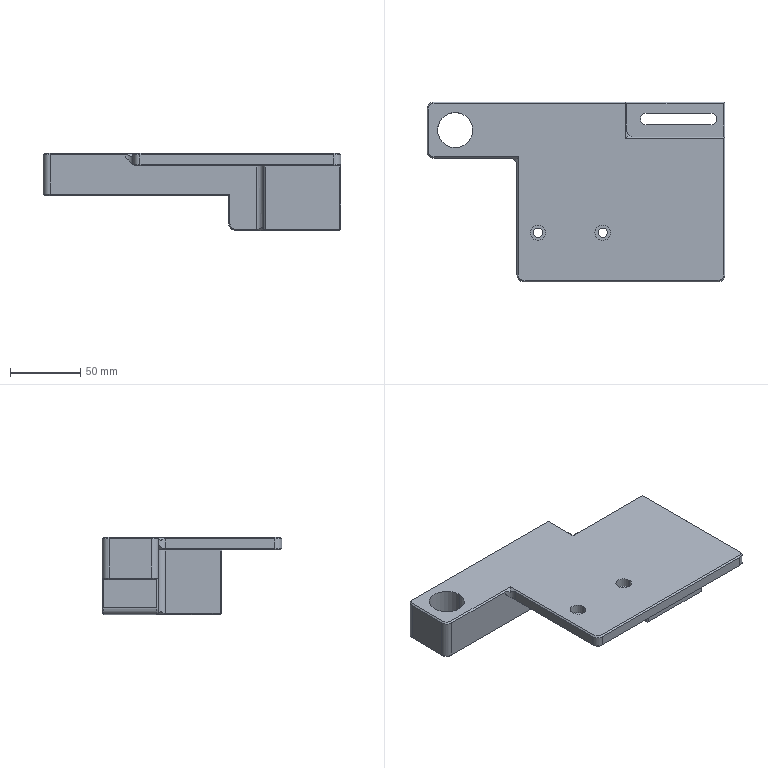NC program | NX | posted with a generic post | part box 212 x 128 x 55 mm
Lines 4578 to 5530 of 8014:
(ZLEVEL_PROFILE_COPY_COPY_COPY_COPY_1 , TOOL : D10)
N9136 T09 M6
N9138 G54
N9140 G17 G0 G90 X-41.719 Y17.8 S2000 M3
N9142 G43 Z30. H9
N9144 Z-0.2
N9146 G94 G1 X-42.585 Y19.3 F1000.
N9148 G3 X-43.451 Y19.8 R1.
N9150 G1 X-46.8 F2000.
N9152 Y16.451
N9154 G3 X-46.3 Y15.585 R1.
N9156 G1 X-44.8 Y14.719
N9158 G0 X-41.519 Y17.6 Z-0.4
N9160 G1 X-42.385 Y19.1 F1000.
N9162 G3 X-43.251 Y19.6 R1.
N9164 G1 X-46.6 F2000.
N9166 Y16.251
N9168 G3 X-46.1 Y15.385 R1.
N9170 G1 X-44.6 Y14.519
N9172 G0 X-41.319 Y17.4 Z-0.6
N9174 G1 X-42.185 Y18.9 F1000.
N9176 G3 X-43.051 Y19.4 R1.
N9178 G1 X-46.4 F2000.
N9180 Y16.051
N9182 G3 X-45.9 Y15.185 R1.
N9184 G1 X-44.4 Y14.319
N9186 G0 X-41.119 Y17.2 Z-0.8
N9188 G1 X-41.985 Y18.7 F1000.
N9190 G3 X-42.851 Y19.2 R1.
N9192 G1 X-46.2 F2000.
N9194 Y15.851
N9196 G3 X-45.7 Y14.985 R1.
N9198 G1 X-44.2 Y14.119
N9200 G0 X-40.919 Y17. Z-1.
N9202 G1 X-41.785 Y18.5 F1000.
N9204 G3 X-42.651 Y19. R1.
N9206 G1 X-45.559 F2000.
N9208 X-46.
N9210 Y15.651
N9212 G3 X-45.5 Y14.785 R1.
N9214 G1 X-44. Y13.919
N9216 G0 X-40.919 Y17. Z-1.2
N9218 G1 X-41.785 Y18.5 F1000.
N9220 G3 X-42.651 Y19. R1.
N9222 G1 X-45.997 F2000.
N9224 X-46. Y18.997
N9226 Y15.651
N9228 G3 X-45.5 Y14.785 R1.
N9230 G1 X-44. Y13.919
N9232 G0 X-40.919 Y17. Z-1.4
N9234 G1 X-41.785 Y18.5 F1000.
N9236 G3 X-42.651 Y19. R1.
N9238 G1 X-45.997 F2000.
N9240 X-46. Y18.997
N9242 Y15.651
N9244 G3 X-45.5 Y14.785 R1.
N9246 G1 X-44. Y13.919
N9248 G0 X-40.919 Y17. Z-1.6
N9250 G1 X-41.785 Y18.5 F1000.
N9252 G3 X-42.651 Y19. R1.
N9254 G1 X-45.997 F2000.
N9256 X-46. Y18.997
N9258 Y15.651
N9260 G3 X-45.5 Y14.785 R1.
N9262 G1 X-44. Y13.919
N9264 G0 X-40.919 Y17. Z-1.8
N9266 G1 X-41.785 Y18.5 F1000.
N9268 G3 X-42.651 Y19. R1.
N9270 G1 X-45.997 F2000.
N9272 X-46. Y18.997
N9274 Y15.651
N9276 G3 X-45.5 Y14.785 R1.
N9278 G1 X-44. Y13.919
N9280 G0 X-40.919 Y17. Z-2.
N9282 G1 X-41.785 Y18.5 F1000.
N9284 G3 X-42.651 Y19. R1.
N9286 G1 X-45.997 F2000.
N9288 X-46. Y18.997
N9290 Y15.651
N9292 G3 X-45.5 Y14.785 R1.
N9294 G1 X-44. Y13.919
N9296 G0 X-40.919 Y17. Z-2.2
N9298 G1 X-41.785 Y18.5 F1000.
N9300 G3 X-42.651 Y19. R1.
N9302 G1 X-45.997 F2000.
N9304 X-46. Y18.997
N9306 Y15.651
N9308 G3 X-45.5 Y14.785 R1.
N9310 G1 X-44. Y13.919
N9312 G0 X-40.919 Y17. Z-2.4
N9314 G1 X-41.785 Y18.5 F1000.
N9316 G3 X-42.651 Y19. R1.
N9318 G1 X-45.997 F2000.
N9320 X-46. Y18.997
N9322 Y15.651
N9324 G3 X-45.5 Y14.785 R1.
N9326 G1 X-44. Y13.919
N9328 G0 X-40.919 Y17. Z-2.6
N9330 G1 X-41.785 Y18.5 F1000.
N9332 G3 X-42.651 Y19. R1.
N9334 G1 X-45.997 F2000.
N9336 X-46. Y18.997
N9338 Y15.651
N9340 G3 X-45.5 Y14.785 R1.
N9342 G1 X-44. Y13.919
N9344 G0 X-40.919 Y17. Z-2.8
N9346 G1 X-41.785 Y18.5 F1000.
N9348 G3 X-42.651 Y19. R1.
N9350 G1 X-45.997 F2000.
N9352 X-46. Y18.997
N9354 Y15.651
N9356 G3 X-45.5 Y14.785 R1.
N9358 G1 X-44. Y13.919
N9360 G0 X-40.919 Y17. Z-3.
N9362 G1 X-41.785 Y18.5 F1000.
N9364 G3 X-42.651 Y19. R1.
N9366 G1 X-45.997 F2000.
N9368 X-46. Y18.997
N9370 Y15.651
N9372 G3 X-45.5 Y14.785 R1.
N9374 G1 X-44. Y13.919
N9376 G0 X-40.919 Y17. Z-3.2
N9378 G1 X-41.785 Y18.5 F1000.
N9380 G3 X-42.651 Y19. R1.
N9382 G1 X-45.997 F2000.
N9384 X-46. Y18.997
N9386 Y15.651
N9388 G3 X-45.5 Y14.785 R1.
N9390 G1 X-44. Y13.919
N9392 G0 X-40.919 Y17. Z-3.4
N9394 G1 X-41.785 Y18.5 F1000.
N9396 G3 X-42.651 Y19. R1.
N9398 G1 X-45.997 F2000.
N9400 X-46. Y18.997
N9402 Y15.651
N9404 G3 X-45.5 Y14.785 R1.
N9406 G1 X-44. Y13.919
N9408 G0 X-40.919 Y17. Z-3.6
N9410 G1 X-41.785 Y18.5 F1000.
N9412 G3 X-42.651 Y19. R1.
N9414 G1 X-45.997 F2000.
N9416 X-46. Y18.997
N9418 Y15.651
N9420 G3 X-45.5 Y14.785 R1.
N9422 G1 X-44. Y13.919
N9424 G0 X-40.919 Y17. Z-3.8
N9426 G1 X-41.785 Y18.5 F1000.
N9428 G3 X-42.651 Y19. R1.
N9430 G1 X-45.997 F2000.
N9432 X-46. Y18.997
N9434 Y15.651
N9436 G3 X-45.5 Y14.785 R1.
N9438 G1 X-44. Y13.919
N9440 G0 X-40.919 Y17. Z-4.
N9442 G1 X-41.785 Y18.5 F1000.
N9444 G3 X-42.651 Y19. R1.
N9446 G1 X-45.997 F2000.
N9448 X-46. Y18.997
N9450 Y15.651
N9452 G3 X-45.5 Y14.785 R1.
N9454 G1 X-44. Y13.919
N9456 G0 X-40.919 Y17. Z-4.2
N9458 G1 X-41.785 Y18.5 F1000.
N9460 G3 X-42.651 Y19. R1.
N9462 G1 X-45.997 F2000.
N9464 X-46. Y18.997
N9466 Y15.651
N9468 G3 X-45.5 Y14.785 R1.
N9470 G1 X-44. Y13.919
N9472 G0 X-40.919 Y17. Z-4.4
N9474 G1 X-41.785 Y18.5 F1000.
N9476 G3 X-42.651 Y19. R1.
N9478 G1 X-45.997 F2000.
N9480 X-46. Y18.997
N9482 Y15.651
N9484 G3 X-45.5 Y14.785 R1.
N9486 G1 X-44. Y13.919
N9488 G0 X-40.919 Y17. Z-4.6
N9490 G1 X-41.785 Y18.5 F1000.
N9492 G3 X-42.651 Y19. R1.
N9494 G1 X-45.997 F2000.
N9496 X-46. Y18.997
N9498 Y15.651
N9500 G3 X-45.5 Y14.785 R1.
N9502 G1 X-44. Y13.919
N9504 G0 X-40.919 Y17. Z-4.8
N9506 G1 X-41.785 Y18.5 F1000.
N9508 G3 X-42.651 Y19. R1.
N9510 G1 X-45.997 F2000.
N9512 X-46. Y18.997
N9514 Y15.651
N9516 G3 X-45.5 Y14.785 R1.
N9518 G1 X-44. Y13.919
N9520 G0 X-40.919 Y17. Z-5.
N9522 G1 X-41.785 Y18.5 F1000.
N9524 G3 X-42.651 Y19. R1.
N9526 G1 X-45.997 F2000.
N9528 X-46. Y18.997
N9530 Y15.651
N9532 G3 X-45.5 Y14.785 R1.
N9534 G1 X-44. Y13.919
N9536 G0 X-40.919 Y17. Z-5.2
N9538 G1 X-41.785 Y18.5 F1000.
N9540 G3 X-42.651 Y19. R1.
N9542 G1 X-45.997 F2000.
N9544 X-46. Y18.997
N9546 Y15.651
N9548 G3 X-45.5 Y14.785 R1.
N9550 G1 X-44. Y13.919
N9552 G0 X-40.919 Y17. Z-5.4
N9554 G1 X-41.785 Y18.5 F1000.
N9556 G3 X-42.651 Y19. R1.
N9558 G1 X-45.997 F2000.
N9560 X-46. Y18.997
N9562 Y15.651
N9564 G3 X-45.5 Y14.785 R1.
N9566 G1 X-44. Y13.919
N9568 G0 X-40.919 Y17. Z-5.6
N9570 G1 X-41.785 Y18.5 F1000.
N9572 G3 X-42.651 Y19. R1.
N9574 G1 X-45.997 F2000.
N9576 X-46. Y18.997
N9578 Y15.651
N9580 G3 X-45.5 Y14.785 R1.
N9582 G1 X-44. Y13.919
N9584 G0 X-40.919 Y17. Z-5.8
N9586 G1 X-41.785 Y18.5 F1000.
N9588 G3 X-42.651 Y19. R1.
N9590 G1 X-45.997 F2000.
N9592 X-46. Y18.997
N9594 Y15.651
N9596 G3 X-45.5 Y14.785 R1.
N9598 G1 X-44. Y13.919
N9600 G0 X-40.919 Y17. Z-6.
N9602 G1 X-41.785 Y18.5 F1000.
N9604 G3 X-42.651 Y19. R1.
N9606 G1 X-45.996 F2000.
N9608 X-46. Y18.996
N9610 Y15.651
N9612 G3 X-45.5 Y14.785 R1.
N9614 G1 X-44. Y13.919
N9616 G0 X-40.919 Y17. Z-6.2
N9618 G1 X-41.785 Y18.5 F1000.
N9620 G3 X-42.651 Y19. R1.
N9622 G1 X-45.996 F2000.
N9624 X-46. Y18.996
N9626 Y15.651
N9628 G3 X-45.5 Y14.785 R1.
N9630 G1 X-44. Y13.919
N9632 G0 X-40.919 Y17. Z-6.4
N9634 G1 X-41.785 Y18.5 F1000.
N9636 G3 X-42.651 Y19. R1.
N9638 G1 X-45.996 F2000.
N9640 X-46. Y18.996
N9642 Y15.651
N9644 G3 X-45.5 Y14.785 R1.
N9646 G1 X-44. Y13.919
N9648 G0 X-40.919 Y17. Z-6.6
N9650 G1 X-41.785 Y18.5 F1000.
N9652 G3 X-42.651 Y19. R1.
N9654 G1 X-45.996 F2000.
N9656 X-46. Y18.996
N9658 Y15.651
N9660 G3 X-45.5 Y14.785 R1.
N9662 G1 X-44. Y13.919
N9664 G0 X-40.919 Y17. Z-6.8
N9666 G1 X-41.785 Y18.5 F1000.
N9668 G3 X-42.651 Y19. R1.
N9670 G1 X-45.996 F2000.
N9672 X-46. Y18.996
N9674 Y15.651
N9676 G3 X-45.5 Y14.785 R1.
N9678 G1 X-44. Y13.919
N9680 G0 X-40.919 Y17. Z-7.
N9682 G1 X-41.785 Y18.5 F1000.
N9684 G3 X-42.651 Y19. R1.
N9686 G1 X-45.996 F2000.
N9688 X-46. Y18.996
N9690 Y15.651
N9692 G3 X-45.5 Y14.785 R1.
N9694 G1 X-44. Y13.919
N9696 G0 X-40.919 Y17. Z-7.2
N9698 G1 X-41.785 Y18.5 F1000.
N9700 G3 X-42.651 Y19. R1.
N9702 G1 X-45.996 F2000.
N9704 X-46. Y18.996
N9706 Y15.651
N9708 G3 X-45.5 Y14.785 R1.
N9710 G1 X-44. Y13.919
N9712 G0 X-40.919 Y17. Z-7.4
N9714 G1 X-41.785 Y18.5 F1000.
N9716 G3 X-42.651 Y19. R1.
N9718 G1 X-45.996 F2000.
N9720 X-46. Y18.996
N9722 Y15.651
N9724 G3 X-45.5 Y14.785 R1.
N9726 G1 X-44. Y13.919
N9728 G0 X-40.919 Y17. Z-7.6
N9730 G1 X-41.785 Y18.5 F1000.
N9732 G3 X-42.651 Y19. R1.
N9734 G1 X-45.996 F2000.
N9736 X-46. Y18.996
N9738 Y15.651
N9740 G3 X-45.5 Y14.785 R1.
N9742 G1 X-44. Y13.919
N9744 G0 X-40.919 Y17. Z-7.8
N9746 G1 X-41.785 Y18.5 F1000.
N9748 G3 X-42.651 Y19. R1.
N9750 G1 X-45.996 F2000.
N9752 X-46. Y18.996
N9754 Y15.651
N9756 G3 X-45.5 Y14.785 R1.
N9758 G1 X-44. Y13.919
N9760 G0 X-40.919 Y17. Z-8.
N9762 G1 X-41.785 Y18.5 F1000.
N9764 G3 X-42.651 Y19. R1.
N9766 G1 X-45.996 F2000.
N9768 X-46. Y18.996
N9770 Y15.651
N9772 G3 X-45.5 Y14.785 R1.
N9774 G1 X-44. Y13.919
N9776 G0 X-40.919 Y17. Z-8.2
N9778 G1 X-41.785 Y18.5 F1000.
N9780 G3 X-42.651 Y19. R1.
N9782 G1 X-45.996 F2000.
N9784 X-46. Y18.996
N9786 Y15.651
N9788 G3 X-45.5 Y14.785 R1.
N9790 G1 X-44. Y13.919
N9792 G0 X-40.919 Y17. Z-8.4
N9794 G1 X-41.785 Y18.5 F1000.
N9796 G3 X-42.651 Y19. R1.
N9798 G1 X-45.996 F2000.
N9800 X-46. Y18.996
N9802 Y15.651
N9804 G3 X-45.5 Y14.785 R1.
N9806 G1 X-44. Y13.919
N9808 G0 X-40.919 Y17. Z-8.6
N9810 G1 X-41.785 Y18.5 F1000.
N9812 G3 X-42.651 Y19. R1.
N9814 G1 X-45.996 F2000.
N9816 X-46. Y18.996
N9818 Y15.651
N9820 G3 X-45.5 Y14.785 R1.
N9822 G1 X-44. Y13.919
N9824 G0 X-40.919 Y17. Z-8.8
N9826 G1 X-41.785 Y18.5 F1000.
N9828 G3 X-42.651 Y19. R1.
N9830 G1 X-45.996 F2000.
N9832 X-46. Y18.996
N9834 Y15.651
N9836 G3 X-45.5 Y14.785 R1.
N9838 G1 X-44. Y13.919
N9840 G0 X-40.919 Y17. Z-9.
N9842 G1 X-41.785 Y18.5 F1000.
N9844 G3 X-42.651 Y19. R1.
N9846 G1 X-45.996 F2000.
N9848 X-46. Y18.996
N9850 Y15.651
N9852 G3 X-45.5 Y14.785 R1.
N9854 G1 X-44. Y13.919
N9856 G0 X-40.919 Y17. Z-9.2
N9858 G1 X-41.785 Y18.5 F1000.
N9860 G3 X-42.651 Y19. R1.
N9862 G1 X-45.996 F2000.
N9864 X-46. Y18.996
N9866 Y15.651
N9868 G3 X-45.5 Y14.785 R1.
N9870 G1 X-44. Y13.919
N9872 G0 X-40.919 Y17. Z-9.4
N9874 G1 X-41.785 Y18.5 F1000.
N9876 G3 X-42.651 Y19. R1.
N9878 G1 X-45.996 F2000.
N9880 X-46. Y18.996
N9882 Y15.651
N9884 G3 X-45.5 Y14.785 R1.
N9886 G1 X-44. Y13.919
N9888 G0 X-40.919 Y17. Z-9.6
N9890 G1 X-41.785 Y18.5 F1000.
N9892 G3 X-42.651 Y19. R1.
N9894 G1 X-45.996 F2000.
N9896 X-46. Y18.996
N9898 Y15.651
N9900 G3 X-45.5 Y14.785 R1.
N9902 G1 X-44. Y13.919
N9904 G0 X-40.919 Y17. Z-9.8
N9906 G1 X-41.785 Y18.5 F1000.
N9908 G3 X-42.651 Y19. R1.
N9910 G1 X-45.996 F2000.
N9912 X-46. Y18.996
N9914 Y15.651
N9916 G3 X-45.5 Y14.785 R1.
N9918 G1 X-44. Y13.919
N9920 G0 X-40.919 Y17. Z-10.
N9922 G1 X-41.785 Y18.5 F1000.
N9924 G3 X-42.651 Y19. R1.
N9926 G1 X-45.996 F2000.
N9928 X-46. Y18.996
N9930 Y15.651
N9932 G3 X-45.5 Y14.785 R1.
N9934 G1 X-44. Y13.919
N9936 G0 X-40.919 Y17. Z-10.2
N9938 G1 X-41.785 Y18.5 F1000.
N9940 G3 X-42.651 Y19. R1.
N9942 G1 X-45.996 F2000.
N9944 X-46. Y18.996
N9946 Y15.651
N9948 G3 X-45.5 Y14.785 R1.
N9950 G1 X-44. Y13.919
N9952 G0 X-40.919 Y17. Z-10.4
N9954 G1 X-41.785 Y18.5 F1000.
N9956 G3 X-42.651 Y19. R1.
N9958 G1 X-45.996 F2000.
N9960 X-46. Y18.996
N9962 Y15.651
N9964 G3 X-45.5 Y14.785 R1.
N9966 G1 X-44. Y13.919
N9968 G0 X-40.919 Y17. Z-10.6
N9970 G1 X-41.785 Y18.5 F1000.
N9972 G3 X-42.651 Y19. R1.
N9974 G1 X-45.996 F2000.
N9976 X-46. Y18.996
N9978 Y15.651
N9980 G3 X-45.5 Y14.785 R1.
N9982 G1 X-44. Y13.919
N9984 G0 X-40.919 Y17. Z-10.8
N9986 G1 X-41.785 Y18.5 F1000.
N9988 G3 X-42.651 Y19. R1.
N9990 G1 X-45.996 F2000.
N9992 X-46. Y18.996
N9994 Y15.651
N9996 G3 X-45.5 Y14.785 R1.
N9998 G1 X-44. Y13.919
N10000 G0 X-40.919 Y17. Z-11.
N10002 G1 X-41.785 Y18.5 F1000.
N10004 G3 X-42.651 Y19. R1.
N10006 G1 X-45.996 F2000.
N10008 X-46. Y18.996
N10010 Y15.651
N10012 G3 X-45.5 Y14.785 R1.
N10014 G1 X-44. Y13.919
N10016 G0 X-40.919 Y17. Z-11.2
N10018 G1 X-41.785 Y18.5 F1000.
N10020 G3 X-42.651 Y19. R1.
N10022 G1 X-45.996 F2000.
N10024 X-46. Y18.996
N10026 Y15.651
N10028 G3 X-45.5 Y14.785 R1.
N10030 G1 X-44. Y13.919
N10032 G0 X-40.919 Y17. Z-11.4
N10034 G1 X-41.785 Y18.5 F1000.
N10036 G3 X-42.651 Y19. R1.
N10038 G1 X-45.996 F2000.
N10040 X-46. Y18.996
N10042 Y15.651
N10044 G3 X-45.5 Y14.785 R1.
N10046 G1 X-44. Y13.919
N10048 G0 X-40.919 Y17. Z-11.6
N10050 G1 X-41.785 Y18.5 F1000.
N10052 G3 X-42.651 Y19. R1.
N10054 G1 X-45.996 F2000.
N10056 X-46. Y18.996
N10058 Y15.651
N10060 G3 X-45.5 Y14.785 R1.
N10062 G1 X-44. Y13.919
N10064 G0 X-40.919 Y17. Z-11.8
N10066 G1 X-41.785 Y18.5 F1000.
N10068 G3 X-42.651 Y19. R1.
N10070 G1 X-45.996 F2000.
N10072 X-46. Y18.996
N10074 Y15.651
N10076 G3 X-45.5 Y14.785 R1.
N10078 G1 X-44. Y13.919
N10080 G0 X-40.919 Y17. Z-12.
N10082 G1 X-41.785 Y18.5 F1000.
N10084 G3 X-42.651 Y19. R1.
N10086 G1 X-45.996 F2000.
N10088 X-46. Y18.996
N10090 Y15.651
N10092 G3 X-45.5 Y14.785 R1.
N10094 G1 X-44. Y13.919
N10096 G0 X-40.919 Y17. Z-12.2
N10098 G1 X-41.785 Y18.5 F1000.
N10100 G3 X-42.651 Y19. R1.
N10102 G1 X-45.996 F2000.
N10104 X-46. Y18.996
N10106 Y15.651
N10108 G3 X-45.5 Y14.785 R1.
N10110 G1 X-44. Y13.919
N10112 G0 X-40.919 Y17. Z-12.4
N10114 G1 X-41.785 Y18.5 F1000.
N10116 G3 X-42.651 Y19. R1.
N10118 G1 X-45.996 F2000.
N10120 X-46. Y18.996
N10122 Y15.651
N10124 G3 X-45.5 Y14.785 R1.
N10126 G1 X-44. Y13.919
N10128 G0 X-40.919 Y17. Z-12.6
N10130 G1 X-41.785 Y18.5 F1000.
N10132 G3 X-42.651 Y19. R1.
N10134 G1 X-45.996 F2000.
N10136 X-46. Y18.996
N10138 Y15.651
N10140 G3 X-45.5 Y14.785 R1.
N10142 G1 X-44. Y13.919
N10144 G0 X-40.919 Y17. Z-12.8
N10146 G1 X-41.785 Y18.5 F1000.
N10148 G3 X-42.651 Y19. R1.
N10150 G1 X-45.996 F2000.
N10152 X-46. Y18.996
N10154 Y15.651
N10156 G3 X-45.5 Y14.785 R1.
N10158 G1 X-44. Y13.919
N10160 G0 X-40.919 Y17. Z-13.
N10162 G1 X-41.785 Y18.5 F1000.
N10164 G3 X-42.651 Y19. R1.
N10166 G1 X-45.996 F2000.
N10168 X-46. Y18.996
N10170 Y15.651
N10172 G3 X-45.5 Y14.785 R1.
N10174 G1 X-44. Y13.919
N10176 G0 X-40.919 Y17. Z-13.2
N10178 G1 X-41.785 Y18.5 F1000.
N10180 G3 X-42.651 Y19. R1.
N10182 G1 X-45.996 F2000.
N10184 X-46. Y18.996
N10186 Y15.651
N10188 G3 X-45.5 Y14.785 R1.
N10190 G1 X-44. Y13.919
N10192 G0 X-40.919 Y17. Z-13.4
N10194 G1 X-41.785 Y18.5 F1000.
N10196 G3 X-42.651 Y19. R1.
N10198 G1 X-45.996 F2000.
N10200 X-46. Y18.996
N10202 Y15.651
N10204 G3 X-45.5 Y14.785 R1.
N10206 G1 X-44. Y13.919
N10208 G0 X-40.919 Y17. Z-13.6
N10210 G1 X-41.785 Y18.5 F1000.
N10212 G3 X-42.651 Y19. R1.
N10214 G1 X-45.996 F2000.
N10216 X-46. Y18.996
N10218 Y15.651
N10220 G3 X-45.5 Y14.785 R1.
N10222 G1 X-44. Y13.919
N10224 G0 X-40.919 Y17. Z-13.8
N10226 G1 X-41.785 Y18.5 F1000.
N10228 G3 X-42.651 Y19. R1.
N10230 G1 X-45.996 F2000.
N10232 X-46. Y18.996
N10234 Y15.651
N10236 G3 X-45.5 Y14.785 R1.
N10238 G1 X-44. Y13.919
N10240 G0 X-40.919 Y17. Z-14.
N10242 G1 X-41.785 Y18.5 F1000.
N10244 G3 X-42.651 Y19. R1.
N10246 G1 X-45.996 F2000.
N10248 X-46. Y18.996
N10250 Y15.651
N10252 G3 X-45.5 Y14.785 R1.
N10254 G1 X-44. Y13.919
N10256 G0 X-40.919 Y17. Z-14.2
N10258 G1 X-41.785 Y18.5 F1000.
N10260 G3 X-42.651 Y19. R1.
N10262 G1 X-45.996 F2000.
N10264 X-46. Y18.996
N10266 Y15.651
N10268 G3 X-45.5 Y14.785 R1.
N10270 G1 X-44. Y13.919
N10272 G0 X-40.919 Y17. Z-14.4
N10274 G1 X-41.785 Y18.5 F1000.
N10276 G3 X-42.651 Y19. R1.
N10278 G1 X-45.996 F2000.
N10280 X-46. Y18.996
N10282 Y15.651
N10284 G3 X-45.5 Y14.785 R1.
N10286 G1 X-44. Y13.919
N10288 G0 X-40.919 Y17. Z-14.6
N10290 G1 X-41.785 Y18.5 F1000.
N10292 G3 X-42.651 Y19. R1.
N10294 G1 X-45.996 F2000.
N10296 X-46. Y18.996
N10298 Y15.651
N10300 G3 X-45.5 Y14.785 R1.
N10302 G1 X-44. Y13.919
N10304 G0 X-40.919 Y17. Z-14.8
N10306 G1 X-41.785 Y18.5 F1000.
N10308 G3 X-42.651 Y19. R1.
N10310 G1 X-45.996 F2000.
N10312 X-46. Y18.996
N10314 Y15.651
N10316 G3 X-45.5 Y14.785 R1.
N10318 G1 X-44. Y13.919
N10320 G0 X-40.919 Y17. Z-15.
N10322 G1 X-41.785 Y18.5 F1000.
N10324 G3 X-42.651 Y19. R1.
N10326 G1 X-45.996 F2000.
N10328 X-46. Y18.996
N10330 Y15.651
N10332 G3 X-45.5 Y14.785 R1.
N10334 G1 X-44. Y13.919
N10336 G0 X-40.919 Y17. Z-15.2
N10338 G1 X-41.785 Y18.5 F1000.
N10340 G3 X-42.651 Y19. R1.
N10342 G1 X-45.996 F2000.
N10344 X-46. Y18.996
N10346 Y15.651
N10348 G3 X-45.5 Y14.785 R1.
N10350 G1 X-44. Y13.919
N10352 G0 X-40.919 Y17. Z-15.4
N10354 G1 X-41.785 Y18.5 F1000.
N10356 G3 X-42.651 Y19. R1.
N10358 G1 X-45.996 F2000.
N10360 X-46. Y18.996
N10362 Y15.651
N10364 G3 X-45.5 Y14.785 R1.
N10366 G1 X-44. Y13.919
N10368 G0 X-40.919 Y17. Z-15.6
N10370 G1 X-41.785 Y18.5 F1000.
N10372 G3 X-42.651 Y19. R1.
N10374 G1 X-45.996 F2000.
N10376 X-46. Y18.996
N10378 Y15.651
N10380 G3 X-45.5 Y14.785 R1.
N10382 G1 X-44. Y13.919
N10384 G0 X-40.919 Y17. Z-15.8
N10386 G1 X-41.785 Y18.5 F1000.
N10388 G3 X-42.651 Y19. R1.
N10390 G1 X-45.996 F2000.
N10392 X-46. Y18.996
N10394 Y15.651
N10396 G3 X-45.5 Y14.785 R1.
N10398 G1 X-44. Y13.919
N10400 G0 X-40.919 Y17. Z-16.
N10402 G1 X-41.785 Y18.5 F1000.
N10404 G3 X-42.651 Y19. R1.
N10406 G1 X-45.996 F2000.
N10408 X-46. Y18.996
N10410 Y15.651
N10412 G3 X-45.5 Y14.785 R1.
N10414 G1 X-44. Y13.919
N10416 G0 X-40.919 Y17. Z-16.2
N10418 G1 X-41.785 Y18.5 F1000.
N10420 G3 X-42.651 Y19. R1.
N10422 G1 X-45.996 F2000.
N10424 X-46. Y18.996
N10426 Y15.651
N10428 G3 X-45.5 Y14.785 R1.
N10430 G1 X-44. Y13.919
N10432 G0 X-40.919 Y17. Z-16.4
N10434 G1 X-41.785 Y18.5 F1000.
N10436 G3 X-42.651 Y19. R1.
N10438 G1 X-45.996 F2000.
N10440 X-46. Y18.996
N10442 Y15.651
N10444 G3 X-45.5 Y14.785 R1.
N10446 G1 X-44. Y13.919
N10448 G0 X-40.919 Y17. Z-16.6
N10450 G1 X-41.785 Y18.5 F1000.
N10452 G3 X-42.651 Y19. R1.
N10454 G1 X-45.996 F2000.
N10456 X-46. Y18.996
N10458 Y15.651
N10460 G3 X-45.5 Y14.785 R1.
N10462 G1 X-44. Y13.919
N10464 G0 X-40.919 Y17. Z-16.8
N10466 G1 X-41.785 Y18.5 F1000.
N10468 G3 X-42.651 Y19. R1.
N10470 G1 X-45.996 F2000.
N10472 X-46. Y18.996
N10474 Y15.651
N10476 G3 X-45.5 Y14.785 R1.
N10478 G1 X-44. Y13.919
N10480 G0 X-40.919 Y17. Z-17.
N10482 G1 X-41.785 Y18.5 F1000.
N10484 G3 X-42.651 Y19. R1.
N10486 G1 X-45.996 F2000.
N10488 X-46. Y18.996
N10490 Y15.651
N10492 G3 X-45.5 Y14.785 R1.
N10494 G1 X-44. Y13.919
N10496 G0 X-40.919 Y17. Z-17.2
N10498 G1 X-41.785 Y18.5 F1000.
N10500 G3 X-42.651 Y19. R1.
N10502 G1 X-45.996 F2000.
N10504 X-46. Y18.996
N10506 Y15.651
N10508 G3 X-45.5 Y14.785 R1.
N10510 G1 X-44. Y13.919
N10512 G0 X-40.919 Y17. Z-17.4
N10514 G1 X-41.785 Y18.5 F1000.
N10516 G3 X-42.651 Y19. R1.
N10518 G1 X-45.996 F2000.
N10520 X-46. Y18.996
N10522 Y15.651
N10524 G3 X-45.5 Y14.785 R1.
N10526 G1 X-44. Y13.919
N10528 G0 X-40.919 Y17. Z-17.6
N10530 G1 X-41.785 Y18.5 F1000.
N10532 G3 X-42.651 Y19. R1.
N10534 G1 X-45.996 F2000.
N10536 X-46. Y18.996
N10538 Y15.651
N10540 G3 X-45.5 Y14.785 R1.
N10542 G1 X-44. Y13.919
N10544 G0 X-40.919 Y17. Z-17.8
N10546 G1 X-41.785 Y18.5 F1000.
N10548 G3 X-42.651 Y19. R1.
N10550 G1 X-45.996 F2000.
N10552 X-46. Y18.996
N10554 Y15.651
N10556 G3 X-45.5 Y14.785 R1.
N10558 G1 X-44. Y13.919
N10560 G0 X-40.919 Y17. Z-18.
N10562 G1 X-41.785 Y18.5 F1000.
N10564 G3 X-42.651 Y19. R1.
N10566 G1 X-45.996 F2000.
N10568 X-46. Y18.996
N10570 Y15.651
N10572 G3 X-45.5 Y14.785 R1.
N10574 G1 X-44. Y13.919
N10576 G0 X-40.919 Y17. Z-18.2
N10578 G1 X-41.785 Y18.5 F1000.
N10580 G3 X-42.651 Y19. R1.
N10582 G1 X-45.996 F2000.
N10584 X-46. Y18.996
N10586 Y15.651
N10588 G3 X-45.5 Y14.785 R1.
N10590 G1 X-44. Y13.919
N10592 G0 X-40.919 Y17. Z-18.4
N10594 G1 X-41.785 Y18.5 F1000.
N10596 G3 X-42.651 Y19. R1.
N10598 G1 X-45.996 F2000.
N10600 X-46. Y18.996
N10602 Y15.651
N10604 G3 X-45.5 Y14.785 R1.
N10606 G1 X-44. Y13.919
N10608 G0 X-40.919 Y17. Z-18.6
N10610 G1 X-41.785 Y18.5 F1000.
N10612 G3 X-42.651 Y19. R1.
N10614 G1 X-45.996 F2000.
N10616 X-46. Y18.996
N10618 Y15.651
N10620 G3 X-45.5 Y14.785 R1.
N10622 G1 X-44. Y13.919
N10624 G0 X-40.919 Y17. Z-18.8
N10626 G1 X-41.785 Y18.5 F1000.
N10628 G3 X-42.651 Y19. R1.
N10630 G1 X-45.996 F2000.
N10632 X-46. Y18.996
N10634 Y15.651
N10636 G3 X-45.5 Y14.785 R1.
N10638 G1 X-44. Y13.919
N10640 G0 X-40.919 Y17. Z-19.
N10642 G1 X-41.785 Y18.5 F1000.
N10644 G3 X-42.651 Y19. R1.
N10646 G1 X-45.996 F2000.
N10648 X-46. Y18.996
N10650 Y15.651
N10652 G3 X-45.5 Y14.785 R1.
N10654 G1 X-44. Y13.919
N10656 G0 X-40.919 Y17. Z-19.2
N10658 G1 X-41.785 Y18.5 F1000.
N10660 G3 X-42.651 Y19. R1.
N10662 G1 X-45.996 F2000.
N10664 X-46. Y18.996
N10666 Y15.651
N10668 G3 X-45.5 Y14.785 R1.
N10670 G1 X-44. Y13.919
N10672 G0 X-40.919 Y17. Z-19.4
N10674 G1 X-41.785 Y18.5 F1000.
N10676 G3 X-42.651 Y19. R1.
N10678 G1 X-45.996 F2000.
N10680 X-46. Y18.996
N10682 Y15.651
N10684 G3 X-45.5 Y14.785 R1.
N10686 G1 X-44. Y13.919
N10688 G0 X-40.919 Y17. Z-19.6
N10690 G1 X-41.785 Y18.5 F1000.
N10692 G3 X-42.651 Y19. R1.
N10694 G1 X-45.996 F2000.
N10696 X-46. Y18.996
N10698 Y15.651
N10700 G3 X-45.5 Y14.785 R1.
N10702 G1 X-44. Y13.919
N10704 G0 X-40.919 Y17. Z-19.8
N10706 G1 X-41.785 Y18.5 F1000.
N10708 G3 X-42.651 Y19. R1.
N10710 G1 X-45.996 F2000.
N10712 X-46. Y18.996
N10714 Y15.651
N10716 G3 X-45.5 Y14.785 R1.
N10718 G1 X-44. Y13.919
N10720 G0 X-40.919 Y17. Z-20.
N10722 G1 X-41.785 Y18.5 F1000.
N10724 G3 X-42.651 Y19. R1.
N10726 G1 X-45.996 F2000.
N10728 X-46. Y18.996
N10730 Y15.651
N10732 G3 X-45.5 Y14.785 R1.
N10734 G1 X-44. Y13.919
N10736 G0 X-40.919 Y17. Z-20.2
N10738 G1 X-41.785 Y18.5 F1000.
N10740 G3 X-42.651 Y19. R1.
N10742 G1 X-45.996 F2000.
N10744 X-46. Y18.996
N10746 Y15.651
N10748 G3 X-45.5 Y14.785 R1.
N10750 G1 X-44. Y13.919
N10752 G0 X-40.919 Y17. Z-20.4
N10754 G1 X-41.785 Y18.5 F1000.
N10756 G3 X-42.651 Y19. R1.
N10758 G1 X-45.996 F2000.
N10760 X-46. Y18.996
N10762 Y15.651
N10764 G3 X-45.5 Y14.785 R1.
N10766 G1 X-44. Y13.919
N10768 G0 X-40.919 Y17. Z-20.6
N10770 G1 X-41.785 Y18.5 F1000.
N10772 G3 X-42.651 Y19. R1.
N10774 G1 X-45.996 F2000.
N10776 X-46. Y18.996
N10778 Y15.651
N10780 G3 X-45.5 Y14.785 R1.
N10782 G1 X-44. Y13.919
N10784 G0 X-40.919 Y17. Z-20.8
N10786 G1 X-41.785 Y18.5 F1000.
N10788 G3 X-42.651 Y19. R1.
N10790 G1 X-45.996 F2000.
N10792 X-46. Y18.996
N10794 Y15.651
N10796 G3 X-45.5 Y14.785 R1.
N10798 G1 X-44. Y13.919
N10800 G0 X-40.919 Y17. Z-21.
N10802 G1 X-41.785 Y18.5 F1000.
N10804 G3 X-42.651 Y19. R1.
N10806 G1 X-45.996 F2000.
N10808 X-46. Y18.996
N10810 Y15.651
N10812 G3 X-45.5 Y14.785 R1.
N10814 G1 X-44. Y13.919
N10816 G0 X-40.919 Y17. Z-21.2
N10818 G1 X-41.785 Y18.5 F1000.
N10820 G3 X-42.651 Y19. R1.
N10822 G1 X-45.996 F2000.
N10824 X-46. Y18.996
N10826 Y15.651
N10828 G3 X-45.5 Y14.785 R1.
N10830 G1 X-44. Y13.919
N10832 G0 X-40.919 Y17. Z-21.4
N10834 G1 X-41.785 Y18.5 F1000.
N10836 G3 X-42.651 Y19. R1.
N10838 G1 X-45.996 F2000.
N10840 X-46. Y18.996
N10842 Y15.651
N10844 G3 X-45.5 Y14.785 R1.
N10846 G1 X-44. Y13.919
N10848 G0 X-40.919 Y17. Z-21.6
N10850 G1 X-41.785 Y18.5 F1000.
N10852 G3 X-42.651 Y19. R1.
N10854 G1 X-45.996 F2000.
N10856 X-46. Y18.996
N10858 Y15.651
N10860 G3 X-45.5 Y14.785 R1.
N10862 G1 X-44. Y13.919
N10864 G0 X-40.919 Y17. Z-21.8
N10866 G1 X-41.785 Y18.5 F1000.
N10868 G3 X-42.651 Y19. R1.
N10870 G1 X-45.996 F2000.
N10872 X-46. Y18.996
N10874 Y15.651
N10876 G3 X-45.5 Y14.785 R1.
N10878 G1 X-44. Y13.919
N10880 G0 X-40.919 Y17. Z-22.
N10882 G1 X-41.785 Y18.5 F1000.
N10884 G3 X-42.651 Y19. R1.
N10886 G1 X-45.996 F2000.
N10888 X-46. Y18.996
N10890 Y15.651
N10892 G3 X-45.5 Y14.785 R1.
N10894 G1 X-44. Y13.919
N10896 G0 X-40.919 Y17. Z-22.2
N10898 G1 X-41.785 Y18.5 F1000.
N10900 G3 X-42.651 Y19. R1.
N10902 G1 X-45.996 F2000.
N10904 X-46. Y18.996
N10906 Y15.651
N10908 G3 X-45.5 Y14.785 R1.
N10910 G1 X-44. Y13.919
N10912 G0 X-40.919 Y17. Z-22.4
N10914 G1 X-41.785 Y18.5 F1000.
N10916 G3 X-42.651 Y19. R1.
N10918 G1 X-45.995 F2000.
N10920 X-46. Y18.995
N10922 Y15.651
N10924 G3 X-45.5 Y14.785 R1.
N10926 G1 X-44. Y13.919
N10928 G0 X-40.919 Y17. Z-22.6
N10930 G1 X-41.785 Y18.5 F1000.
N10932 G3 X-42.651 Y19. R1.
N10934 G1 X-45.995 F2000.
N10936 X-46. Y18.995
N10938 Y15.651
N10940 G3 X-45.5 Y14.785 R1.
N10942 G1 X-44. Y13.919
N10944 G0 X-40.919 Y17. Z-22.8
N10946 G1 X-41.785 Y18.5 F1000.
N10948 G3 X-42.651 Y19. R1.
N10950 G1 X-45.995 F2000.
N10952 X-46. Y18.995
N10954 Y15.651
N10956 G3 X-45.5 Y14.785 R1.
N10958 G1 X-44. Y13.919
N10960 G0 X-40.919 Y17. Z-23.
N10962 G1 X-41.785 Y18.5 F1000.
N10964 G3 X-42.651 Y19. R1.
N10966 G1 X-45.995 F2000.
N10968 X-46. Y18.995
N10970 Y15.651
N10972 G3 X-45.5 Y14.785 R1.
N10974 G1 X-44. Y13.919
N10976 G0 X-40.919 Y17. Z-23.2
N10978 G1 X-41.785 Y18.5 F1000.
N10980 G3 X-42.651 Y19. R1.
N10982 G1 X-45.995 F2000.
N10984 X-46. Y18.995
N10986 Y15.651
N10988 G3 X-45.5 Y14.785 R1.
N10990 G1 X-44. Y13.919
N10992 G0 X-40.919 Y17. Z-23.4
N10994 G1 X-41.785 Y18.5 F1000.
N10996 G3 X-42.651 Y19. R1.
N10998 G1 X-45.995 F2000.
N11000 X-46. Y18.995
N11002 Y15.651
N11004 G3 X-45.5 Y14.785 R1.
N11006 G1 X-44. Y13.919
N11008 G0 X-40.919 Y17. Z-23.6
N11010 G1 X-41.785 Y18.5 F1000.
N11012 G3 X-42.651 Y19. R1.
N11014 G1 X-45.995 F2000.
N11016 X-46. Y18.995
N11018 Y15.651
N11020 G3 X-45.5 Y14.785 R1.
N11022 G1 X-44. Y13.919
N11024 G0 X-40.919 Y17. Z-23.8
N11026 G1 X-41.785 Y18.5 F1000.
N11028 G3 X-42.651 Y19. R1.
N11030 G1 X-45.995 F2000.
N11032 X-46. Y18.995
N11034 Y15.651